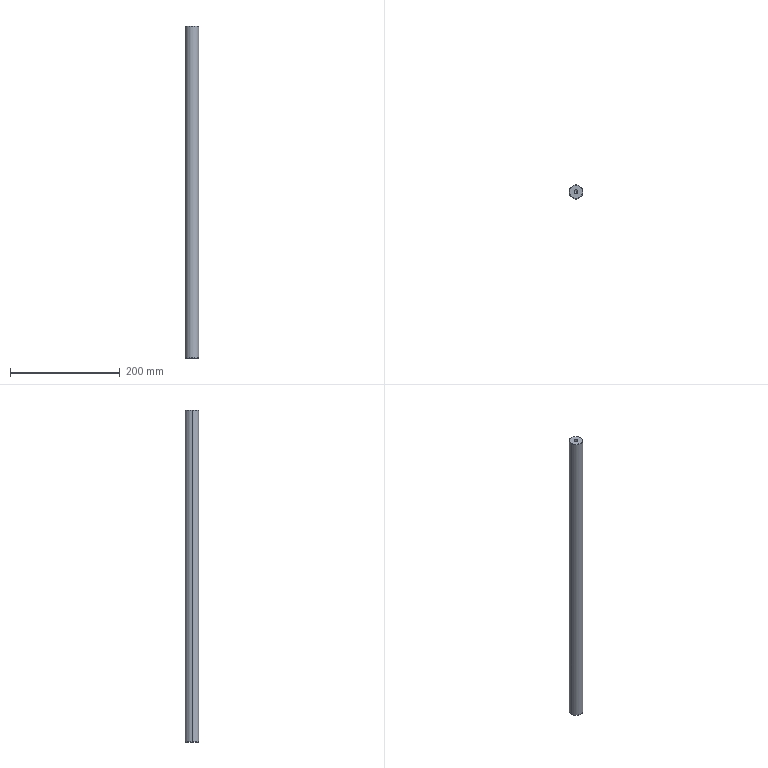Part | SolidWorks | features HoleWzd 2, Chamfer 1, Extrusion 1 | 1 solid | 16 faces | box 25 x 25 x 605 mm | volume 295385 mm3 | cone 8 | cylinder 6 | plane 2 | commonest cylinder face diameters 6.8 x4 25 x2
STEP:
#1=CARTESIAN_POINT('',(-3.4,0.,585.25));
#2=VERTEX_POINT('',#1);
#3=CARTESIAN_POINT('',(3.4,0.,585.25));
#4=VERTEX_POINT('',#3);
#5=CARTESIAN_POINT('',(0.,0.,585.25));
#6=DIRECTION('',(0.,0.,1.));
#7=DIRECTION('',(1.,0.,0.));
#8=AXIS2_PLACEMENT_3D('',#5,#6,#7);
#9=CIRCLE('',#8,3.4);
#10=EDGE_CURVE('',#2,#4,#9,.T.);
#11=ORIENTED_EDGE('',*,*,#10,.F.);
#12=CARTESIAN_POINT('',(-3.4,0.,605.));
#13=VERTEX_POINT('',#12);
#14=CARTESIAN_POINT('',(-3.4,0.,605.));
#15=DIRECTION('',(0.,0.,1.));
#16=VECTOR('',#15,1000.);
#17=LINE('',#14,#16);
#18=EDGE_CURVE('',#2,#13,#17,.T.);
#19=ORIENTED_EDGE('',*,*,#18,.T.);
#20=CARTESIAN_POINT('',(3.4,0.,605.));
#21=VERTEX_POINT('',#20);
#22=CARTESIAN_POINT('',(0.,0.,605.));
#23=DIRECTION('',(0.,0.,1.));
#24=DIRECTION('',(1.,0.,0.));
#25=AXIS2_PLACEMENT_3D('',#22,#23,#24);
#26=CIRCLE('',#25,3.4);
#27=EDGE_CURVE('',#13,#21,#26,.T.);
#28=ORIENTED_EDGE('',*,*,#27,.T.);
#29=CARTESIAN_POINT('',(3.4,0.,605.));
#30=DIRECTION('',(0.,0.,1.));
#31=VECTOR('',#30,1000.);
#32=LINE('',#29,#31);
#33=EDGE_CURVE('',#4,#21,#32,.T.);
#34=ORIENTED_EDGE('',*,*,#33,.F.);
#35=EDGE_LOOP('',(#11,#19,#28,#34));
#36=FACE_OUTER_BOUND('',#35,.T.);
#37=CARTESIAN_POINT('',(0.,0.,605.));
#38=DIRECTION('',(0.,0.,1.));
#39=DIRECTION('',(1.,0.,0.));
#40=AXIS2_PLACEMENT_3D('',#37,#38,#39);
#41=CYLINDRICAL_SURFACE('',#40,3.4);
#42=ADVANCED_FACE('',(#36),#41,.F.);
#43=CARTESIAN_POINT('',(0.,0.,583.207));
#44=VERTEX_POINT('',#43);
#45=CARTESIAN_POINT('',(3.4,0.,585.25));
#46=DIRECTION('',(0.8572,0.,0.515));
#47=VECTOR('',#46,1000.);
#48=LINE('',#45,#47);
#49=EDGE_CURVE('',#44,#4,#48,.T.);
#50=ORIENTED_EDGE('',*,*,#49,.F.);
#51=CARTESIAN_POINT('',(-3.4,0.,585.25));
#52=DIRECTION('',(-0.8572,0.,0.515));
#53=VECTOR('',#52,1000.);
#54=LINE('',#51,#53);
#55=EDGE_CURVE('',#44,#2,#54,.T.);
#56=ORIENTED_EDGE('',*,*,#55,.T.);
#57=ORIENTED_EDGE('',*,*,#10,.T.);
#58=EDGE_LOOP('',(#50,#56,#57));
#59=FACE_OUTER_BOUND('',#58,.T.);
#60=CARTESIAN_POINT('',(0.,0.,585.25));
#61=DIRECTION('',(0.,0.,1.));
#62=DIRECTION('',(1.,0.,0.));
#63=AXIS2_PLACEMENT_3D('',#60,#61,#62);
#64=CONICAL_SURFACE('',#63,3.4,1.03);
#65=ADVANCED_FACE('',(#59),#64,.F.);
#66=CARTESIAN_POINT('',(-12.,0.,0.));
#67=VERTEX_POINT('',#66);
#68=CARTESIAN_POINT('',(12.,0.,0.));
#69=VERTEX_POINT('',#68);
#70=CARTESIAN_POINT('',(0.,0.,0.));
#71=DIRECTION('',(0.,0.,-1.));
#72=DIRECTION('',(1.,0.,0.));
#73=AXIS2_PLACEMENT_3D('',#70,#71,#72);
#74=CIRCLE('',#73,12.);
#75=EDGE_CURVE('',#67,#69,#74,.T.);
#76=ORIENTED_EDGE('',*,*,#75,.F.);
#77=CARTESIAN_POINT('',(-12.5,0.,0.5));
#78=VERTEX_POINT('',#77);
#79=CARTESIAN_POINT('',(-12.5,0.,0.5));
#80=DIRECTION('',(-0.7071,0.,0.7071));
#81=VECTOR('',#80,1000.);
#82=LINE('',#79,#81);
#83=EDGE_CURVE('',#67,#78,#82,.T.);
#84=ORIENTED_EDGE('',*,*,#83,.T.);
#85=CARTESIAN_POINT('',(12.5,0.,0.5));
#86=VERTEX_POINT('',#85);
#87=CARTESIAN_POINT('',(0.,0.,0.5));
#88=DIRECTION('',(0.,0.,1.));
#89=DIRECTION('',(1.,0.,0.));
#90=AXIS2_PLACEMENT_3D('',#87,#88,#89);
#91=CIRCLE('',#90,12.5);
#92=EDGE_CURVE('',#86,#78,#91,.T.);
#93=ORIENTED_EDGE('',*,*,#92,.F.);
#94=CARTESIAN_POINT('',(12.5,0.,0.5));
#95=DIRECTION('',(0.7071,0.,0.7071));
#96=VECTOR('',#95,1000.);
#97=LINE('',#94,#96);
#98=EDGE_CURVE('',#69,#86,#97,.T.);
#99=ORIENTED_EDGE('',*,*,#98,.F.);
#100=EDGE_LOOP('',(#76,#84,#93,#99));
#101=FACE_OUTER_BOUND('',#100,.T.);
#102=CARTESIAN_POINT('',(0.,0.,0.5));
#103=DIRECTION('',(0.,0.,1.));
#104=DIRECTION('',(1.,0.,0.));
#105=AXIS2_PLACEMENT_3D('',#102,#103,#104);
#106=CONICAL_SURFACE('',#105,12.5,0.7854);
#107=ADVANCED_FACE('',(#101),#106,.T.);
#108=CARTESIAN_POINT('',(12.,0.,605.));
#109=VERTEX_POINT('',#108);
#110=CARTESIAN_POINT('',(-12.,0.,605.));
#111=VERTEX_POINT('',#110);
#112=CARTESIAN_POINT('',(0.,0.,605.));
#113=DIRECTION('',(0.,0.,1.));
#114=DIRECTION('',(1.,0.,0.));
#115=AXIS2_PLACEMENT_3D('',#112,#113,#114);
#116=CIRCLE('',#115,12.);
#117=EDGE_CURVE('',#109,#111,#116,.T.);
#118=ORIENTED_EDGE('',*,*,#117,.F.);
#119=CARTESIAN_POINT('',(12.5,0.,604.5));
#120=VERTEX_POINT('',#119);
#121=CARTESIAN_POINT('',(12.,0.,605.));
#122=DIRECTION('',(0.7071,0.,-0.7071));
#123=VECTOR('',#122,1000.);
#124=LINE('',#121,#123);
#125=EDGE_CURVE('',#109,#120,#124,.T.);
#126=ORIENTED_EDGE('',*,*,#125,.T.);
#127=CARTESIAN_POINT('',(-12.5,0.,604.5));
#128=VERTEX_POINT('',#127);
#129=CARTESIAN_POINT('',(0.,0.,604.5));
#130=DIRECTION('',(0.,0.,-1.));
#131=DIRECTION('',(1.,0.,0.));
#132=AXIS2_PLACEMENT_3D('',#129,#130,#131);
#133=CIRCLE('',#132,12.5);
#134=EDGE_CURVE('',#128,#120,#133,.T.);
#135=ORIENTED_EDGE('',*,*,#134,.F.);
#136=CARTESIAN_POINT('',(-12.,0.,605.));
#137=DIRECTION('',(-0.7071,0.,-0.7071));
#138=VECTOR('',#137,1000.);
#139=LINE('',#136,#138);
#140=EDGE_CURVE('',#111,#128,#139,.T.);
#141=ORIENTED_EDGE('',*,*,#140,.F.);
#142=EDGE_LOOP('',(#118,#126,#135,#141));
#143=FACE_OUTER_BOUND('',#142,.T.);
#144=CARTESIAN_POINT('',(0.,0.,605.));
#145=DIRECTION('',(0.,0.,-1.));
#146=DIRECTION('',(-1.,0.,0.));
#147=AXIS2_PLACEMENT_3D('',#144,#145,#146);
#148=CONICAL_SURFACE('',#147,12.,0.7854);
#149=ADVANCED_FACE('',(#143),#148,.T.);
#150=CARTESIAN_POINT('',(3.4,0.,22.25));
#151=VERTEX_POINT('',#150);
#152=CARTESIAN_POINT('',(-3.4,0.,22.25));
#153=VERTEX_POINT('',#152);
#154=CARTESIAN_POINT('',(0.,0.,22.25));
#155=DIRECTION('',(0.,0.,-1.));
#156=DIRECTION('',(-1.,0.,0.));
#157=AXIS2_PLACEMENT_3D('',#154,#155,#156);
#158=CIRCLE('',#157,3.4);
#159=EDGE_CURVE('',#151,#153,#158,.T.);
#160=ORIENTED_EDGE('',*,*,#159,.F.);
#161=CARTESIAN_POINT('',(3.4,0.,0.));
#162=VERTEX_POINT('',#161);
#163=CARTESIAN_POINT('',(3.4,0.,0.));
#164=DIRECTION('',(0.,0.,-1.));
#165=VECTOR('',#164,1000.);
#166=LINE('',#163,#165);
#167=EDGE_CURVE('',#151,#162,#166,.T.);
#168=ORIENTED_EDGE('',*,*,#167,.T.);
#169=CARTESIAN_POINT('',(-3.4,0.,0.));
#170=VERTEX_POINT('',#169);
#171=CARTESIAN_POINT('',(0.,0.,0.));
#172=DIRECTION('',(0.,0.,-1.));
#173=DIRECTION('',(-1.,0.,0.));
#174=AXIS2_PLACEMENT_3D('',#171,#172,#173);
#175=CIRCLE('',#174,3.4);
#176=EDGE_CURVE('',#162,#170,#175,.T.);
#177=ORIENTED_EDGE('',*,*,#176,.T.);
#178=CARTESIAN_POINT('',(-3.4,0.,0.));
#179=DIRECTION('',(0.,0.,-1.));
#180=VECTOR('',#179,1000.);
#181=LINE('',#178,#180);
#182=EDGE_CURVE('',#153,#170,#181,.T.);
#183=ORIENTED_EDGE('',*,*,#182,.F.);
#184=EDGE_LOOP('',(#160,#168,#177,#183));
#185=FACE_OUTER_BOUND('',#184,.T.);
#186=CARTESIAN_POINT('',(0.,0.,0.));
#187=DIRECTION('',(0.,0.,-1.));
#188=DIRECTION('',(-1.,0.,0.));
#189=AXIS2_PLACEMENT_3D('',#186,#187,#188);
#190=CYLINDRICAL_SURFACE('',#189,3.4);
#191=ADVANCED_FACE('',(#185),#190,.F.);
#192=CARTESIAN_POINT('',(0.,0.,24.293));
#193=VERTEX_POINT('',#192);
#194=CARTESIAN_POINT('',(-3.4,0.,22.25));
#195=DIRECTION('',(-0.8572,0.,-0.515));
#196=VECTOR('',#195,1000.);
#197=LINE('',#194,#196);
#198=EDGE_CURVE('',#193,#153,#197,.T.);
#199=ORIENTED_EDGE('',*,*,#198,.F.);
#200=CARTESIAN_POINT('',(3.4,0.,22.25));
#201=DIRECTION('',(0.8572,0.,-0.515));
#202=VECTOR('',#201,1000.);
#203=LINE('',#200,#202);
#204=EDGE_CURVE('',#193,#151,#203,.T.);
#205=ORIENTED_EDGE('',*,*,#204,.T.);
#206=ORIENTED_EDGE('',*,*,#159,.T.);
#207=EDGE_LOOP('',(#199,#205,#206));
#208=FACE_OUTER_BOUND('',#207,.T.);
#209=CARTESIAN_POINT('',(0.,0.,22.25));
#210=DIRECTION('',(0.,0.,-1.));
#211=DIRECTION('',(-1.,0.,0.));
#212=AXIS2_PLACEMENT_3D('',#209,#210,#211);
#213=CONICAL_SURFACE('',#212,3.4,1.03);
#214=ADVANCED_FACE('',(#208),#213,.F.);
#215=ORIENTED_EDGE('',*,*,#134,.T.);
#216=CARTESIAN_POINT('',(12.5,0.,605.));
#217=DIRECTION('',(0.,0.,-1.));
#218=VECTOR('',#217,1000.);
#219=LINE('',#216,#218);
#220=EDGE_CURVE('',#120,#86,#219,.T.);
#221=ORIENTED_EDGE('',*,*,#220,.T.);
#222=ORIENTED_EDGE('',*,*,#92,.T.);
#223=CARTESIAN_POINT('',(-12.5,0.,605.));
#224=DIRECTION('',(0.,0.,-1.));
#225=VECTOR('',#224,1000.);
#226=LINE('',#223,#225);
#227=EDGE_CURVE('',#128,#78,#226,.T.);
#228=ORIENTED_EDGE('',*,*,#227,.F.);
#229=EDGE_LOOP('',(#215,#221,#222,#228));
#230=FACE_OUTER_BOUND('',#229,.T.);
#231=CARTESIAN_POINT('',(0.,0.,605.));
#232=DIRECTION('',(0.,0.,-1.));
#233=DIRECTION('',(-1.,0.,0.));
#234=AXIS2_PLACEMENT_3D('',#231,#232,#233);
#235=CYLINDRICAL_SURFACE('',#234,12.5);
#236=ADVANCED_FACE('',(#230),#235,.T.);
#237=ORIENTED_EDGE('',*,*,#220,.F.);
#238=CARTESIAN_POINT('',(0.,0.,604.5));
#239=DIRECTION('',(0.,0.,-1.));
#240=DIRECTION('',(1.,0.,0.));
#241=AXIS2_PLACEMENT_3D('',#238,#239,#240);
#242=CIRCLE('',#241,12.5);
#243=EDGE_CURVE('',#120,#128,#242,.T.);
#244=ORIENTED_EDGE('',*,*,#243,.T.);
#245=ORIENTED_EDGE('',*,*,#227,.T.);
#246=CARTESIAN_POINT('',(0.,0.,0.5));
#247=DIRECTION('',(0.,0.,1.));
#248=DIRECTION('',(1.,0.,0.));
#249=AXIS2_PLACEMENT_3D('',#246,#247,#248);
#250=CIRCLE('',#249,12.5);
#251=EDGE_CURVE('',#78,#86,#250,.T.);
#252=ORIENTED_EDGE('',*,*,#251,.T.);
#253=EDGE_LOOP('',(#237,#244,#245,#252));
#254=FACE_OUTER_BOUND('',#253,.T.);
#255=CARTESIAN_POINT('',(0.,0.,605.));
#256=DIRECTION('',(0.,0.,-1.));
#257=DIRECTION('',(-1.,0.,0.));
#258=AXIS2_PLACEMENT_3D('',#255,#256,#257);
#259=CYLINDRICAL_SURFACE('',#258,12.5);
#260=ADVANCED_FACE('',(#254),#259,.T.);
#261=CARTESIAN_POINT('',(0.,0.,605.));
#262=DIRECTION('',(0.,0.,1.));
#263=DIRECTION('',(1.,0.,0.));
#264=AXIS2_PLACEMENT_3D('',#261,#262,#263);
#265=CIRCLE('',#264,3.4);
#266=EDGE_CURVE('',#21,#13,#265,.T.);
#267=ORIENTED_EDGE('',*,*,#266,.F.);
#268=ORIENTED_EDGE('',*,*,#27,.F.);
#269=EDGE_LOOP('',(#267,#268));
#270=FACE_BOUND('',#269,.T.);
#271=CARTESIAN_POINT('',(0.,0.,605.));
#272=DIRECTION('',(0.,0.,1.));
#273=DIRECTION('',(1.,0.,0.));
#274=AXIS2_PLACEMENT_3D('',#271,#272,#273);
#275=CIRCLE('',#274,12.);
#276=EDGE_CURVE('',#111,#109,#275,.T.);
#277=ORIENTED_EDGE('',*,*,#276,.T.);
#278=ORIENTED_EDGE('',*,*,#117,.T.);
#279=EDGE_LOOP('',(#277,#278));
#280=FACE_OUTER_BOUND('',#279,.T.);
#281=CARTESIAN_POINT('',(0.,0.,605.));
#282=DIRECTION('',(0.,0.,1.));
#283=DIRECTION('',(1.,0.,0.));
#284=AXIS2_PLACEMENT_3D('',#281,#282,#283);
#285=PLANE('',#284);
#286=ADVANCED_FACE('',(#270,#280),#285,.T.);
#287=CARTESIAN_POINT('',(0.,0.,0.));
#288=DIRECTION('',(0.,0.,-1.));
#289=DIRECTION('',(1.,0.,0.));
#290=AXIS2_PLACEMENT_3D('',#287,#288,#289);
#291=CIRCLE('',#290,12.);
#292=EDGE_CURVE('',#69,#67,#291,.T.);
#293=ORIENTED_EDGE('',*,*,#292,.T.);
#294=ORIENTED_EDGE('',*,*,#75,.T.);
#295=EDGE_LOOP('',(#293,#294));
#296=FACE_OUTER_BOUND('',#295,.T.);
#297=CARTESIAN_POINT('',(0.,0.,0.));
#298=DIRECTION('',(0.,0.,-1.));
#299=DIRECTION('',(-1.,0.,0.));
#300=AXIS2_PLACEMENT_3D('',#297,#298,#299);
#301=CIRCLE('',#300,3.4);
#302=EDGE_CURVE('',#170,#162,#301,.T.);
#303=ORIENTED_EDGE('',*,*,#302,.F.);
#304=ORIENTED_EDGE('',*,*,#176,.F.);
#305=EDGE_LOOP('',(#303,#304));
#306=FACE_BOUND('',#305,.T.);
#307=CARTESIAN_POINT('',(0.,0.,0.));
#308=DIRECTION('',(0.,0.,1.));
#309=DIRECTION('',(1.,0.,0.));
#310=AXIS2_PLACEMENT_3D('',#307,#308,#309);
#311=PLANE('',#310);
#312=ADVANCED_FACE('',(#296,#306),#311,.F.);
#313=ORIENTED_EDGE('',*,*,#204,.F.);
#314=ORIENTED_EDGE('',*,*,#198,.T.);
#315=CARTESIAN_POINT('',(0.,0.,22.25));
#316=DIRECTION('',(0.,0.,-1.));
#317=DIRECTION('',(-1.,0.,0.));
#318=AXIS2_PLACEMENT_3D('',#315,#316,#317);
#319=CIRCLE('',#318,3.4);
#320=EDGE_CURVE('',#153,#151,#319,.T.);
#321=ORIENTED_EDGE('',*,*,#320,.T.);
#322=EDGE_LOOP('',(#313,#314,#321));
#323=FACE_OUTER_BOUND('',#322,.T.);
#324=CARTESIAN_POINT('',(0.,0.,22.25));
#325=DIRECTION('',(0.,0.,-1.));
#326=DIRECTION('',(-1.,0.,0.));
#327=AXIS2_PLACEMENT_3D('',#324,#325,#326);
#328=CONICAL_SURFACE('',#327,3.4,1.03);
#329=ADVANCED_FACE('',(#323),#328,.F.);
#330=ORIENTED_EDGE('',*,*,#167,.F.);
#331=ORIENTED_EDGE('',*,*,#320,.F.);
#332=ORIENTED_EDGE('',*,*,#182,.T.);
#333=ORIENTED_EDGE('',*,*,#302,.T.);
#334=EDGE_LOOP('',(#330,#331,#332,#333));
#335=FACE_OUTER_BOUND('',#334,.T.);
#336=CARTESIAN_POINT('',(0.,0.,0.));
#337=DIRECTION('',(0.,0.,-1.));
#338=DIRECTION('',(-1.,0.,0.));
#339=AXIS2_PLACEMENT_3D('',#336,#337,#338);
#340=CYLINDRICAL_SURFACE('',#339,3.4);
#341=ADVANCED_FACE('',(#335),#340,.F.);
#342=ORIENTED_EDGE('',*,*,#125,.F.);
#343=ORIENTED_EDGE('',*,*,#276,.F.);
#344=ORIENTED_EDGE('',*,*,#140,.T.);
#345=ORIENTED_EDGE('',*,*,#243,.F.);
#346=EDGE_LOOP('',(#342,#343,#344,#345));
#347=FACE_OUTER_BOUND('',#346,.T.);
#348=CARTESIAN_POINT('',(0.,0.,605.));
#349=DIRECTION('',(0.,0.,-1.));
#350=DIRECTION('',(-1.,0.,0.));
#351=AXIS2_PLACEMENT_3D('',#348,#349,#350);
#352=CONICAL_SURFACE('',#351,12.,0.7854);
#353=ADVANCED_FACE('',(#347),#352,.T.);
#354=ORIENTED_EDGE('',*,*,#83,.F.);
#355=ORIENTED_EDGE('',*,*,#292,.F.);
#356=ORIENTED_EDGE('',*,*,#98,.T.);
#357=ORIENTED_EDGE('',*,*,#251,.F.);
#358=EDGE_LOOP('',(#354,#355,#356,#357));
#359=FACE_OUTER_BOUND('',#358,.T.);
#360=CARTESIAN_POINT('',(0.,0.,0.5));
#361=DIRECTION('',(0.,0.,1.));
#362=DIRECTION('',(1.,0.,0.));
#363=AXIS2_PLACEMENT_3D('',#360,#361,#362);
#364=CONICAL_SURFACE('',#363,12.5,0.7854);
#365=ADVANCED_FACE('',(#359),#364,.T.);
#366=ORIENTED_EDGE('',*,*,#55,.F.);
#367=ORIENTED_EDGE('',*,*,#49,.T.);
#368=CARTESIAN_POINT('',(0.,0.,585.25));
#369=DIRECTION('',(0.,0.,1.));
#370=DIRECTION('',(1.,0.,0.));
#371=AXIS2_PLACEMENT_3D('',#368,#369,#370);
#372=CIRCLE('',#371,3.4);
#373=EDGE_CURVE('',#4,#2,#372,.T.);
#374=ORIENTED_EDGE('',*,*,#373,.T.);
#375=EDGE_LOOP('',(#366,#367,#374));
#376=FACE_OUTER_BOUND('',#375,.T.);
#377=CARTESIAN_POINT('',(0.,0.,585.25));
#378=DIRECTION('',(0.,0.,1.));
#379=DIRECTION('',(1.,0.,0.));
#380=AXIS2_PLACEMENT_3D('',#377,#378,#379);
#381=CONICAL_SURFACE('',#380,3.4,1.03);
#382=ADVANCED_FACE('',(#376),#381,.F.);
#383=ORIENTED_EDGE('',*,*,#18,.F.);
#384=ORIENTED_EDGE('',*,*,#373,.F.);
#385=ORIENTED_EDGE('',*,*,#33,.T.);
#386=ORIENTED_EDGE('',*,*,#266,.T.);
#387=EDGE_LOOP('',(#383,#384,#385,#386));
#388=FACE_OUTER_BOUND('',#387,.T.);
#389=CARTESIAN_POINT('',(0.,0.,605.));
#390=DIRECTION('',(0.,0.,1.));
#391=DIRECTION('',(1.,0.,0.));
#392=AXIS2_PLACEMENT_3D('',#389,#390,#391);
#393=CYLINDRICAL_SURFACE('',#392,3.4);
#394=ADVANCED_FACE('',(#388),#393,.F.);
#395=CLOSED_SHELL('',(#42,#65,#107,#149,#191,#214,#236,#260,#286,#312,#329,#341,#353,#365,#382,#394));
#396=MANIFOLD_SOLID_BREP('',#395);
#397=CARTESIAN_POINT('',(0.,0.,0.));
#398=DIRECTION('',(0.,0.,1.));
#399=DIRECTION('',(1.,0.,0.));
#400=AXIS2_PLACEMENT_3D('',#397,#398,#399);
#401=(LENGTH_UNIT()NAMED_UNIT(*)SI_UNIT(.MILLI.,.METRE.));
#402=UNCERTAINTY_MEASURE_WITH_UNIT(LENGTH_MEASURE(0.00001),#401,'','');
#403=(NAMED_UNIT(*)PLANE_ANGLE_UNIT()SI_UNIT($,.RADIAN.));
#404=(NAMED_UNIT(*)SI_UNIT($,.STERADIAN.)SOLID_ANGLE_UNIT());
#405=(GEOMETRIC_REPRESENTATION_CONTEXT(3)GLOBAL_UNCERTAINTY_ASSIGNED_CONTEXT((#402))GLOBAL_UNIT_ASSIGNED_CONTEXT((#401,#403,#404))REPRESENTATION_CONTEXT('',''));
#406=ADVANCED_BREP_SHAPE_REPRESENTATION('',(#396,#400),#405);